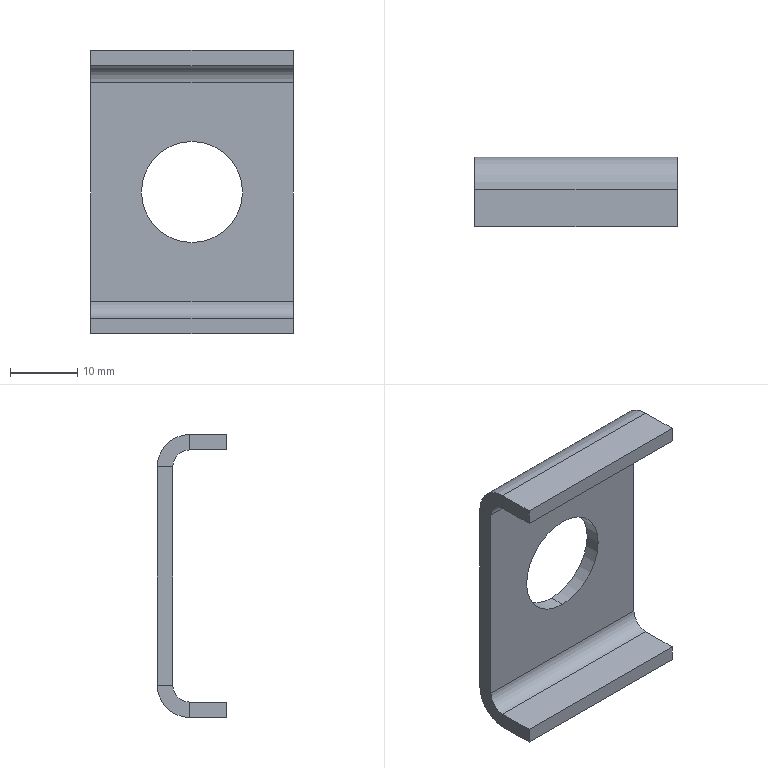Part | SolidWorks | features FlatPattern 1, ICE 1, SMBaseFlange 1, SheetMetal 1 | 1 solid | 24 faces | box 30 x 10.3 x 42 mm | volume 3379 mm3 | plane 18 | cylinder 6 | commonest cylinder face diameters 5 x2 9.6 x2 15 x2
STEP:
#1=CARTESIAN_POINT('',(15.,8.,-13.5));
#2=VERTEX_POINT('',#1);
#3=CARTESIAN_POINT('',(15.,8.,-28.5));
#4=VERTEX_POINT('',#3);
#5=CARTESIAN_POINT('',(15.,8.,-21.));
#6=DIRECTION('',(0.,-1.,0.));
#7=DIRECTION('',(0.,0.,1.));
#8=AXIS2_PLACEMENT_3D('',#5,#6,#7);
#9=CIRCLE('',#8,7.5);
#10=EDGE_CURVE('',#2,#4,#9,.T.);
#11=ORIENTED_EDGE('',*,*,#10,.T.);
#12=CARTESIAN_POINT('',(15.,10.3,-28.5));
#13=VERTEX_POINT('',#12);
#14=CARTESIAN_POINT('',(15.,-0.001,-28.5));
#15=DIRECTION('',(0.,1.,0.));
#16=VECTOR('',#15,1000.);
#17=LINE('',#14,#16);
#18=EDGE_CURVE('',#4,#13,#17,.T.);
#19=ORIENTED_EDGE('',*,*,#18,.T.);
#20=CARTESIAN_POINT('',(15.,10.3,-13.5));
#21=VERTEX_POINT('',#20);
#22=CARTESIAN_POINT('',(15.,10.3,-21.));
#23=DIRECTION('',(0.,1.,0.));
#24=DIRECTION('',(0.,0.,1.));
#25=AXIS2_PLACEMENT_3D('',#22,#23,#24);
#26=CIRCLE('',#25,7.5);
#27=EDGE_CURVE('',#13,#21,#26,.T.);
#28=ORIENTED_EDGE('',*,*,#27,.T.);
#29=CARTESIAN_POINT('',(15.,-0.001,-13.5));
#30=DIRECTION('',(0.,1.,0.));
#31=VECTOR('',#30,1000.);
#32=LINE('',#29,#31);
#33=EDGE_CURVE('',#2,#21,#32,.T.);
#34=ORIENTED_EDGE('',*,*,#33,.F.);
#35=EDGE_LOOP('',(#11,#19,#28,#34));
#36=FACE_OUTER_BOUND('',#35,.T.);
#37=CARTESIAN_POINT('',(15.,-0.001,-21.));
#38=DIRECTION('',(0.,1.,0.));
#39=DIRECTION('',(0.,0.,1.));
#40=AXIS2_PLACEMENT_3D('',#37,#38,#39);
#41=CYLINDRICAL_SURFACE('',#40,7.5);
#42=ADVANCED_FACE('',(#36),#41,.F.);
#43=CARTESIAN_POINT('',(30.,10.3,-4.8));
#44=VERTEX_POINT('',#43);
#45=CARTESIAN_POINT('',(30.,8.,-4.8));
#46=VERTEX_POINT('',#45);
#47=CARTESIAN_POINT('',(30.,10.3,-4.8));
#48=DIRECTION('',(0.,-1.,0.));
#49=VECTOR('',#48,1000.);
#50=LINE('',#47,#49);
#51=EDGE_CURVE('',#44,#46,#50,.T.);
#52=ORIENTED_EDGE('',*,*,#51,.F.);
#53=CARTESIAN_POINT('',(30.,5.5,0.));
#54=VERTEX_POINT('',#53);
#55=CARTESIAN_POINT('',(30.,5.5,-4.8));
#56=DIRECTION('',(-1.,0.,0.));
#57=DIRECTION('',(0.,0.,-1.));
#58=AXIS2_PLACEMENT_3D('',#55,#56,#57);
#59=CIRCLE('',#58,4.8);
#60=EDGE_CURVE('',#54,#44,#59,.T.);
#61=ORIENTED_EDGE('',*,*,#60,.F.);
#62=CARTESIAN_POINT('',(30.,5.5,-2.3));
#63=VERTEX_POINT('',#62);
#64=CARTESIAN_POINT('',(30.,5.5,-2.3));
#65=DIRECTION('',(0.,0.,1.));
#66=VECTOR('',#65,1000.);
#67=LINE('',#64,#66);
#68=EDGE_CURVE('',#63,#54,#67,.T.);
#69=ORIENTED_EDGE('',*,*,#68,.F.);
#70=CARTESIAN_POINT('',(30.,5.5,-4.8));
#71=DIRECTION('',(-1.,0.,0.));
#72=DIRECTION('',(0.,0.,-1.));
#73=AXIS2_PLACEMENT_3D('',#70,#71,#72);
#74=CIRCLE('',#73,2.5);
#75=EDGE_CURVE('',#63,#46,#74,.T.);
#76=ORIENTED_EDGE('',*,*,#75,.T.);
#77=EDGE_LOOP('',(#52,#61,#69,#76));
#78=FACE_OUTER_BOUND('',#77,.T.);
#79=CARTESIAN_POINT('',(30.,10.3,-4.8));
#80=DIRECTION('',(1.,0.,0.));
#81=DIRECTION('',(0.,0.,-1.));
#82=AXIS2_PLACEMENT_3D('',#79,#80,#81);
#83=PLANE('',#82);
#84=ADVANCED_FACE('',(#78),#83,.T.);
#85=CARTESIAN_POINT('',(30.,10.3,-37.2));
#86=VERTEX_POINT('',#85);
#87=CARTESIAN_POINT('',(30.,10.3,0.));
#88=DIRECTION('',(0.,0.,-1.));
#89=VECTOR('',#88,1000.);
#90=LINE('',#87,#89);
#91=EDGE_CURVE('',#44,#86,#90,.T.);
#92=ORIENTED_EDGE('',*,*,#91,.F.);
#93=ORIENTED_EDGE('',*,*,#51,.T.);
#94=CARTESIAN_POINT('',(30.,8.,-37.2));
#95=VERTEX_POINT('',#94);
#96=CARTESIAN_POINT('',(30.,8.,0.));
#97=DIRECTION('',(0.,0.,-1.));
#98=VECTOR('',#97,1000.);
#99=LINE('',#96,#98);
#100=EDGE_CURVE('',#46,#95,#99,.T.);
#101=ORIENTED_EDGE('',*,*,#100,.T.);
#102=CARTESIAN_POINT('',(30.,8.,-37.2));
#103=DIRECTION('',(0.,1.,0.));
#104=VECTOR('',#103,1000.);
#105=LINE('',#102,#104);
#106=EDGE_CURVE('',#95,#86,#105,.T.);
#107=ORIENTED_EDGE('',*,*,#106,.T.);
#108=EDGE_LOOP('',(#92,#93,#101,#107));
#109=FACE_OUTER_BOUND('',#108,.T.);
#110=CARTESIAN_POINT('',(30.,5.5,-2.3));
#111=DIRECTION('',(1.,0.,0.));
#112=DIRECTION('',(0.,0.,-1.));
#113=AXIS2_PLACEMENT_3D('',#110,#111,#112);
#114=PLANE('',#113);
#115=ADVANCED_FACE('',(#109),#114,.T.);
#116=CARTESIAN_POINT('',(0.,5.5,0.));
#117=VERTEX_POINT('',#116);
#118=CARTESIAN_POINT('',(0.,5.5,-2.3));
#119=VERTEX_POINT('',#118);
#120=CARTESIAN_POINT('',(0.,5.5,0.));
#121=DIRECTION('',(0.,0.,-1.));
#122=VECTOR('',#121,1000.);
#123=LINE('',#120,#122);
#124=EDGE_CURVE('',#117,#119,#123,.T.);
#125=ORIENTED_EDGE('',*,*,#124,.F.);
#126=CARTESIAN_POINT('',(0.,10.3,-4.8));
#127=VERTEX_POINT('',#126);
#128=CARTESIAN_POINT('',(0.,5.5,-4.8));
#129=DIRECTION('',(-1.,0.,0.));
#130=DIRECTION('',(0.,0.,-1.));
#131=AXIS2_PLACEMENT_3D('',#128,#129,#130);
#132=CIRCLE('',#131,4.8);
#133=EDGE_CURVE('',#117,#127,#132,.T.);
#134=ORIENTED_EDGE('',*,*,#133,.T.);
#135=CARTESIAN_POINT('',(0.,8.,-4.8));
#136=VERTEX_POINT('',#135);
#137=CARTESIAN_POINT('',(0.,8.,-4.8));
#138=DIRECTION('',(0.,1.,0.));
#139=VECTOR('',#138,1000.);
#140=LINE('',#137,#139);
#141=EDGE_CURVE('',#136,#127,#140,.T.);
#142=ORIENTED_EDGE('',*,*,#141,.F.);
#143=CARTESIAN_POINT('',(0.,5.5,-4.8));
#144=DIRECTION('',(-1.,0.,0.));
#145=DIRECTION('',(0.,0.,-1.));
#146=AXIS2_PLACEMENT_3D('',#143,#144,#145);
#147=CIRCLE('',#146,2.5);
#148=EDGE_CURVE('',#119,#136,#147,.T.);
#149=ORIENTED_EDGE('',*,*,#148,.F.);
#150=EDGE_LOOP('',(#125,#134,#142,#149));
#151=FACE_OUTER_BOUND('',#150,.T.);
#152=CARTESIAN_POINT('',(0.,5.5,0.));
#153=DIRECTION('',(-1.,0.,0.));
#154=DIRECTION('',(0.,0.,1.));
#155=AXIS2_PLACEMENT_3D('',#152,#153,#154);
#156=PLANE('',#155);
#157=ADVANCED_FACE('',(#151),#156,.T.);
#158=CARTESIAN_POINT('',(0.,0.,0.));
#159=VERTEX_POINT('',#158);
#160=CARTESIAN_POINT('',(0.,0.,0.));
#161=DIRECTION('',(0.,1.,0.));
#162=VECTOR('',#161,1000.);
#163=LINE('',#160,#162);
#164=EDGE_CURVE('',#159,#117,#163,.T.);
#165=ORIENTED_EDGE('',*,*,#164,.T.);
#166=ORIENTED_EDGE('',*,*,#124,.T.);
#167=CARTESIAN_POINT('',(0.,0.,-2.3));
#168=VERTEX_POINT('',#167);
#169=CARTESIAN_POINT('',(0.,0.,-2.3));
#170=DIRECTION('',(0.,1.,0.));
#171=VECTOR('',#170,1000.);
#172=LINE('',#169,#171);
#173=EDGE_CURVE('',#168,#119,#172,.T.);
#174=ORIENTED_EDGE('',*,*,#173,.F.);
#175=CARTESIAN_POINT('',(0.,0.,-2.3));
#176=DIRECTION('',(0.,0.,1.));
#177=VECTOR('',#176,1000.);
#178=LINE('',#175,#177);
#179=EDGE_CURVE('',#168,#159,#178,.T.);
#180=ORIENTED_EDGE('',*,*,#179,.T.);
#181=EDGE_LOOP('',(#165,#166,#174,#180));
#182=FACE_OUTER_BOUND('',#181,.T.);
#183=CARTESIAN_POINT('',(0.,8.,-4.8));
#184=DIRECTION('',(-1.,0.,0.));
#185=DIRECTION('',(0.,0.,1.));
#186=AXIS2_PLACEMENT_3D('',#183,#184,#185);
#187=PLANE('',#186);
#188=ADVANCED_FACE('',(#182),#187,.T.);
#189=CARTESIAN_POINT('',(30.,5.5,-42.));
#190=VERTEX_POINT('',#189);
#191=CARTESIAN_POINT('',(30.,5.5,-39.7));
#192=VERTEX_POINT('',#191);
#193=CARTESIAN_POINT('',(30.,5.5,-42.));
#194=DIRECTION('',(0.,0.,1.));
#195=VECTOR('',#194,1000.);
#196=LINE('',#193,#195);
#197=EDGE_CURVE('',#190,#192,#196,.T.);
#198=ORIENTED_EDGE('',*,*,#197,.F.);
#199=CARTESIAN_POINT('',(30.,5.5,-37.2));
#200=DIRECTION('',(-1.,0.,0.));
#201=DIRECTION('',(0.,0.,-1.));
#202=AXIS2_PLACEMENT_3D('',#199,#200,#201);
#203=CIRCLE('',#202,4.8);
#204=EDGE_CURVE('',#86,#190,#203,.T.);
#205=ORIENTED_EDGE('',*,*,#204,.F.);
#206=ORIENTED_EDGE('',*,*,#106,.F.);
#207=CARTESIAN_POINT('',(30.,5.5,-37.2));
#208=DIRECTION('',(-1.,0.,0.));
#209=DIRECTION('',(0.,0.,-1.));
#210=AXIS2_PLACEMENT_3D('',#207,#208,#209);
#211=CIRCLE('',#210,2.5);
#212=EDGE_CURVE('',#95,#192,#211,.T.);
#213=ORIENTED_EDGE('',*,*,#212,.T.);
#214=EDGE_LOOP('',(#198,#205,#206,#213));
#215=FACE_OUTER_BOUND('',#214,.T.);
#216=CARTESIAN_POINT('',(30.,5.5,-42.));
#217=DIRECTION('',(1.,0.,0.));
#218=DIRECTION('',(0.,0.,-1.));
#219=AXIS2_PLACEMENT_3D('',#216,#217,#218);
#220=PLANE('',#219);
#221=ADVANCED_FACE('',(#215),#220,.T.);
#222=CARTESIAN_POINT('',(30.,0.,-42.));
#223=VERTEX_POINT('',#222);
#224=CARTESIAN_POINT('',(30.,10.3,-42.));
#225=DIRECTION('',(0.,-1.,0.));
#226=VECTOR('',#225,1000.);
#227=LINE('',#224,#226);
#228=EDGE_CURVE('',#190,#223,#227,.T.);
#229=ORIENTED_EDGE('',*,*,#228,.F.);
#230=ORIENTED_EDGE('',*,*,#197,.T.);
#231=CARTESIAN_POINT('',(30.,0.,-39.7));
#232=VERTEX_POINT('',#231);
#233=CARTESIAN_POINT('',(30.,10.3,-39.7));
#234=DIRECTION('',(0.,-1.,0.));
#235=VECTOR('',#234,1000.);
#236=LINE('',#233,#235);
#237=EDGE_CURVE('',#192,#232,#236,.T.);
#238=ORIENTED_EDGE('',*,*,#237,.T.);
#239=CARTESIAN_POINT('',(30.,0.,-42.));
#240=DIRECTION('',(0.,0.,1.));
#241=VECTOR('',#240,1000.);
#242=LINE('',#239,#241);
#243=EDGE_CURVE('',#223,#232,#242,.T.);
#244=ORIENTED_EDGE('',*,*,#243,.F.);
#245=EDGE_LOOP('',(#229,#230,#238,#244));
#246=FACE_OUTER_BOUND('',#245,.T.);
#247=CARTESIAN_POINT('',(30.,8.,-37.2));
#248=DIRECTION('',(1.,0.,0.));
#249=DIRECTION('',(0.,0.,-1.));
#250=AXIS2_PLACEMENT_3D('',#247,#248,#249);
#251=PLANE('',#250);
#252=ADVANCED_FACE('',(#246),#251,.T.);
#253=CARTESIAN_POINT('',(0.,10.3,-37.2));
#254=VERTEX_POINT('',#253);
#255=CARTESIAN_POINT('',(0.,8.,-37.2));
#256=VERTEX_POINT('',#255);
#257=CARTESIAN_POINT('',(0.,10.3,-37.2));
#258=DIRECTION('',(0.,-1.,0.));
#259=VECTOR('',#258,1000.);
#260=LINE('',#257,#259);
#261=EDGE_CURVE('',#254,#256,#260,.T.);
#262=ORIENTED_EDGE('',*,*,#261,.F.);
#263=CARTESIAN_POINT('',(0.,5.5,-42.));
#264=VERTEX_POINT('',#263);
#265=CARTESIAN_POINT('',(0.,5.5,-37.2));
#266=DIRECTION('',(-1.,0.,0.));
#267=DIRECTION('',(0.,0.,-1.));
#268=AXIS2_PLACEMENT_3D('',#265,#266,#267);
#269=CIRCLE('',#268,4.8);
#270=EDGE_CURVE('',#254,#264,#269,.T.);
#271=ORIENTED_EDGE('',*,*,#270,.T.);
#272=CARTESIAN_POINT('',(0.,5.5,-39.7));
#273=VERTEX_POINT('',#272);
#274=CARTESIAN_POINT('',(0.,5.5,-39.7));
#275=DIRECTION('',(0.,0.,-1.));
#276=VECTOR('',#275,1000.);
#277=LINE('',#274,#276);
#278=EDGE_CURVE('',#273,#264,#277,.T.);
#279=ORIENTED_EDGE('',*,*,#278,.F.);
#280=CARTESIAN_POINT('',(0.,5.5,-37.2));
#281=DIRECTION('',(-1.,0.,0.));
#282=DIRECTION('',(0.,0.,-1.));
#283=AXIS2_PLACEMENT_3D('',#280,#281,#282);
#284=CIRCLE('',#283,2.5);
#285=EDGE_CURVE('',#256,#273,#284,.T.);
#286=ORIENTED_EDGE('',*,*,#285,.F.);
#287=EDGE_LOOP('',(#262,#271,#279,#286));
#288=FACE_OUTER_BOUND('',#287,.T.);
#289=CARTESIAN_POINT('',(0.,10.3,-37.2));
#290=DIRECTION('',(-1.,0.,0.));
#291=DIRECTION('',(0.,0.,1.));
#292=AXIS2_PLACEMENT_3D('',#289,#290,#291);
#293=PLANE('',#292);
#294=ADVANCED_FACE('',(#288),#293,.T.);
#295=CARTESIAN_POINT('',(0.,10.3,0.));
#296=DIRECTION('',(0.,0.,-1.));
#297=VECTOR('',#296,1000.);
#298=LINE('',#295,#297);
#299=EDGE_CURVE('',#127,#254,#298,.T.);
#300=ORIENTED_EDGE('',*,*,#299,.T.);
#301=ORIENTED_EDGE('',*,*,#261,.T.);
#302=CARTESIAN_POINT('',(0.,8.,0.));
#303=DIRECTION('',(0.,0.,-1.));
#304=VECTOR('',#303,1000.);
#305=LINE('',#302,#304);
#306=EDGE_CURVE('',#136,#256,#305,.T.);
#307=ORIENTED_EDGE('',*,*,#306,.F.);
#308=ORIENTED_EDGE('',*,*,#141,.T.);
#309=EDGE_LOOP('',(#300,#301,#307,#308));
#310=FACE_OUTER_BOUND('',#309,.T.);
#311=CARTESIAN_POINT('',(0.,5.5,-39.7));
#312=DIRECTION('',(-1.,0.,0.));
#313=DIRECTION('',(0.,0.,1.));
#314=AXIS2_PLACEMENT_3D('',#311,#312,#313);
#315=PLANE('',#314);
#316=ADVANCED_FACE('',(#310),#315,.T.);
#317=CARTESIAN_POINT('',(0.,0.,-39.7));
#318=VERTEX_POINT('',#317);
#319=CARTESIAN_POINT('',(0.,10.3,-39.7));
#320=DIRECTION('',(0.,-1.,0.));
#321=VECTOR('',#320,1000.);
#322=LINE('',#319,#321);
#323=EDGE_CURVE('',#273,#318,#322,.T.);
#324=ORIENTED_EDGE('',*,*,#323,.T.);
#325=CARTESIAN_POINT('',(30.,0.,-39.7));
#326=DIRECTION('',(-1.,0.,0.));
#327=VECTOR('',#326,1000.);
#328=LINE('',#325,#327);
#329=EDGE_CURVE('',#232,#318,#328,.T.);
#330=ORIENTED_EDGE('',*,*,#329,.F.);
#331=ORIENTED_EDGE('',*,*,#237,.F.);
#332=CARTESIAN_POINT('',(30.,5.5,-39.7));
#333=DIRECTION('',(-1.,0.,0.));
#334=VECTOR('',#333,1000.);
#335=LINE('',#332,#334);
#336=EDGE_CURVE('',#192,#273,#335,.T.);
#337=ORIENTED_EDGE('',*,*,#336,.T.);
#338=EDGE_LOOP('',(#324,#330,#331,#337));
#339=FACE_OUTER_BOUND('',#338,.T.);
#340=CARTESIAN_POINT('',(30.,10.3,-39.7));
#341=DIRECTION('',(0.,0.,-1.));
#342=DIRECTION('',(-1.,0.,0.));
#343=AXIS2_PLACEMENT_3D('',#340,#341,#342);
#344=PLANE('',#343);
#345=ADVANCED_FACE('',(#339),#344,.F.);
#346=CARTESIAN_POINT('',(0.,0.,-42.));
#347=VERTEX_POINT('',#346);
#348=CARTESIAN_POINT('',(0.,0.,-42.));
#349=DIRECTION('',(0.,0.,1.));
#350=VECTOR('',#349,1000.);
#351=LINE('',#348,#350);
#352=EDGE_CURVE('',#347,#318,#351,.T.);
#353=ORIENTED_EDGE('',*,*,#352,.F.);
#354=CARTESIAN_POINT('',(30.,0.,-42.));
#355=DIRECTION('',(-1.,0.,0.));
#356=VECTOR('',#355,1000.);
#357=LINE('',#354,#356);
#358=EDGE_CURVE('',#223,#347,#357,.T.);
#359=ORIENTED_EDGE('',*,*,#358,.F.);
#360=ORIENTED_EDGE('',*,*,#243,.T.);
#361=ORIENTED_EDGE('',*,*,#329,.T.);
#362=EDGE_LOOP('',(#353,#359,#360,#361));
#363=FACE_OUTER_BOUND('',#362,.T.);
#364=CARTESIAN_POINT('',(30.,0.,-42.));
#365=DIRECTION('',(0.,-1.,0.));
#366=DIRECTION('',(0.,0.,-1.));
#367=AXIS2_PLACEMENT_3D('',#364,#365,#366);
#368=PLANE('',#367);
#369=ADVANCED_FACE('',(#363),#368,.T.);
#370=CARTESIAN_POINT('',(0.,10.3,-42.));
#371=DIRECTION('',(0.,-1.,0.));
#372=VECTOR('',#371,1000.);
#373=LINE('',#370,#372);
#374=EDGE_CURVE('',#264,#347,#373,.T.);
#375=ORIENTED_EDGE('',*,*,#374,.F.);
#376=CARTESIAN_POINT('',(30.,5.5,-42.));
#377=DIRECTION('',(-1.,0.,0.));
#378=VECTOR('',#377,1000.);
#379=LINE('',#376,#378);
#380=EDGE_CURVE('',#190,#264,#379,.T.);
#381=ORIENTED_EDGE('',*,*,#380,.F.);
#382=ORIENTED_EDGE('',*,*,#228,.T.);
#383=ORIENTED_EDGE('',*,*,#358,.T.);
#384=EDGE_LOOP('',(#375,#381,#382,#383));
#385=FACE_OUTER_BOUND('',#384,.T.);
#386=CARTESIAN_POINT('',(30.,10.3,-42.));
#387=DIRECTION('',(0.,0.,-1.));
#388=DIRECTION('',(-1.,0.,0.));
#389=AXIS2_PLACEMENT_3D('',#386,#387,#388);
#390=PLANE('',#389);
#391=ADVANCED_FACE('',(#385),#390,.T.);
#392=ORIENTED_EDGE('',*,*,#270,.F.);
#393=CARTESIAN_POINT('',(30.,10.3,-37.2));
#394=DIRECTION('',(-1.,0.,0.));
#395=VECTOR('',#394,1000.);
#396=LINE('',#393,#395);
#397=EDGE_CURVE('',#86,#254,#396,.T.);
#398=ORIENTED_EDGE('',*,*,#397,.F.);
#399=ORIENTED_EDGE('',*,*,#204,.T.);
#400=ORIENTED_EDGE('',*,*,#380,.T.);
#401=EDGE_LOOP('',(#392,#398,#399,#400));
#402=FACE_OUTER_BOUND('',#401,.T.);
#403=CARTESIAN_POINT('',(30.,5.5,-37.2));
#404=DIRECTION('',(-1.,0.,0.));
#405=DIRECTION('',(0.,0.,1.));
#406=AXIS2_PLACEMENT_3D('',#403,#404,#405);
#407=CYLINDRICAL_SURFACE('',#406,4.8);
#408=ADVANCED_FACE('',(#402),#407,.T.);
#409=CARTESIAN_POINT('',(15.,10.3,-21.));
#410=DIRECTION('',(0.,1.,0.));
#411=DIRECTION('',(0.,0.,1.));
#412=AXIS2_PLACEMENT_3D('',#409,#410,#411);
#413=CIRCLE('',#412,7.5);
#414=EDGE_CURVE('',#21,#13,#413,.T.);
#415=ORIENTED_EDGE('',*,*,#414,.F.);
#416=ORIENTED_EDGE('',*,*,#27,.F.);
#417=EDGE_LOOP('',(#415,#416));
#418=FACE_BOUND('',#417,.T.);
#419=ORIENTED_EDGE('',*,*,#299,.F.);
#420=CARTESIAN_POINT('',(30.,10.3,-4.8));
#421=DIRECTION('',(-1.,0.,0.));
#422=VECTOR('',#421,1000.);
#423=LINE('',#420,#422);
#424=EDGE_CURVE('',#44,#127,#423,.T.);
#425=ORIENTED_EDGE('',*,*,#424,.F.);
#426=ORIENTED_EDGE('',*,*,#91,.T.);
#427=ORIENTED_EDGE('',*,*,#397,.T.);
#428=EDGE_LOOP('',(#419,#425,#426,#427));
#429=FACE_OUTER_BOUND('',#428,.T.);
#430=CARTESIAN_POINT('',(30.,10.3,0.));
#431=DIRECTION('',(0.,1.,0.));
#432=DIRECTION('',(0.,0.,1.));
#433=AXIS2_PLACEMENT_3D('',#430,#431,#432);
#434=PLANE('',#433);
#435=ADVANCED_FACE('',(#418,#429),#434,.T.);
#436=ORIENTED_EDGE('',*,*,#133,.F.);
#437=CARTESIAN_POINT('',(30.,5.5,0.));
#438=DIRECTION('',(-1.,0.,0.));
#439=VECTOR('',#438,1000.);
#440=LINE('',#437,#439);
#441=EDGE_CURVE('',#54,#117,#440,.T.);
#442=ORIENTED_EDGE('',*,*,#441,.F.);
#443=ORIENTED_EDGE('',*,*,#60,.T.);
#444=ORIENTED_EDGE('',*,*,#424,.T.);
#445=EDGE_LOOP('',(#436,#442,#443,#444));
#446=FACE_OUTER_BOUND('',#445,.T.);
#447=CARTESIAN_POINT('',(30.,5.5,-4.8));
#448=DIRECTION('',(-1.,0.,0.));
#449=DIRECTION('',(0.,0.,1.));
#450=AXIS2_PLACEMENT_3D('',#447,#448,#449);
#451=CYLINDRICAL_SURFACE('',#450,4.8);
#452=ADVANCED_FACE('',(#446),#451,.T.);
#453=ORIENTED_EDGE('',*,*,#164,.F.);
#454=CARTESIAN_POINT('',(30.,0.,0.));
#455=VERTEX_POINT('',#454);
#456=CARTESIAN_POINT('',(30.,0.,0.));
#457=DIRECTION('',(-1.,0.,0.));
#458=VECTOR('',#457,1000.);
#459=LINE('',#456,#458);
#460=EDGE_CURVE('',#455,#159,#459,.T.);
#461=ORIENTED_EDGE('',*,*,#460,.F.);
#462=CARTESIAN_POINT('',(30.,0.,0.));
#463=DIRECTION('',(0.,1.,0.));
#464=VECTOR('',#463,1000.);
#465=LINE('',#462,#464);
#466=EDGE_CURVE('',#455,#54,#465,.T.);
#467=ORIENTED_EDGE('',*,*,#466,.T.);
#468=ORIENTED_EDGE('',*,*,#441,.T.);
#469=EDGE_LOOP('',(#453,#461,#467,#468));
#470=FACE_OUTER_BOUND('',#469,.T.);
#471=CARTESIAN_POINT('',(30.,0.,0.));
#472=DIRECTION('',(0.,0.,1.));
#473=DIRECTION('',(1.,0.,0.));
#474=AXIS2_PLACEMENT_3D('',#471,#472,#473);
#475=PLANE('',#474);
#476=ADVANCED_FACE('',(#470),#475,.T.);
#477=ORIENTED_EDGE('',*,*,#179,.F.);
#478=CARTESIAN_POINT('',(30.,0.,-2.3));
#479=VERTEX_POINT('',#478);
#480=CARTESIAN_POINT('',(30.,0.,-2.3));
#481=DIRECTION('',(-1.,0.,0.));
#482=VECTOR('',#481,1000.);
#483=LINE('',#480,#482);
#484=EDGE_CURVE('',#479,#168,#483,.T.);
#485=ORIENTED_EDGE('',*,*,#484,.F.);
#486=CARTESIAN_POINT('',(30.,0.,-2.3));
#487=DIRECTION('',(0.,0.,1.));
#488=VECTOR('',#487,1000.);
#489=LINE('',#486,#488);
#490=EDGE_CURVE('',#479,#455,#489,.T.);
#491=ORIENTED_EDGE('',*,*,#490,.T.);
#492=ORIENTED_EDGE('',*,*,#460,.T.);
#493=EDGE_LOOP('',(#477,#485,#491,#492));
#494=FACE_OUTER_BOUND('',#493,.T.);
#495=CARTESIAN_POINT('',(30.,0.,-2.3));
#496=DIRECTION('',(0.,-1.,0.));
#497=DIRECTION('',(0.,0.,-1.));
#498=AXIS2_PLACEMENT_3D('',#495,#496,#497);
#499=PLANE('',#498);
#500=ADVANCED_FACE('',(#494),#499,.T.);
#501=ORIENTED_EDGE('',*,*,#173,.T.);
#502=CARTESIAN_POINT('',(30.,5.5,-2.3));
#503=DIRECTION('',(-1.,0.,0.));
#504=VECTOR('',#503,1000.);
#505=LINE('',#502,#504);
#506=EDGE_CURVE('',#63,#119,#505,.T.);
#507=ORIENTED_EDGE('',*,*,#506,.F.);
#508=CARTESIAN_POINT('',(30.,0.,-2.3));
#509=DIRECTION('',(0.,1.,0.));
#510=VECTOR('',#509,1000.);
#511=LINE('',#508,#510);
#512=EDGE_CURVE('',#479,#63,#511,.T.);
#513=ORIENTED_EDGE('',*,*,#512,.F.);
#514=ORIENTED_EDGE('',*,*,#484,.T.);
#515=EDGE_LOOP('',(#501,#507,#513,#514));
#516=FACE_OUTER_BOUND('',#515,.T.);
#517=CARTESIAN_POINT('',(30.,0.,-2.3));
#518=DIRECTION('',(0.,0.,1.));
#519=DIRECTION('',(1.,0.,0.));
#520=AXIS2_PLACEMENT_3D('',#517,#518,#519);
#521=PLANE('',#520);
#522=ADVANCED_FACE('',(#516),#521,.F.);
#523=ORIENTED_EDGE('',*,*,#148,.T.);
#524=CARTESIAN_POINT('',(30.,8.,-4.8));
#525=DIRECTION('',(-1.,0.,0.));
#526=VECTOR('',#525,1000.);
#527=LINE('',#524,#526);
#528=EDGE_CURVE('',#46,#136,#527,.T.);
#529=ORIENTED_EDGE('',*,*,#528,.F.);
#530=ORIENTED_EDGE('',*,*,#75,.F.);
#531=ORIENTED_EDGE('',*,*,#506,.T.);
#532=EDGE_LOOP('',(#523,#529,#530,#531));
#533=FACE_OUTER_BOUND('',#532,.T.);
#534=CARTESIAN_POINT('',(30.,5.5,-4.8));
#535=DIRECTION('',(-1.,0.,0.));
#536=DIRECTION('',(0.,0.,1.));
#537=AXIS2_PLACEMENT_3D('',#534,#535,#536);
#538=CYLINDRICAL_SURFACE('',#537,2.5);
#539=ADVANCED_FACE('',(#533),#538,.F.);
#540=ORIENTED_EDGE('',*,*,#10,.F.);
#541=CARTESIAN_POINT('',(15.,8.,-21.));
#542=DIRECTION('',(0.,-1.,0.));
#543=DIRECTION('',(0.,0.,1.));
#544=AXIS2_PLACEMENT_3D('',#541,#542,#543);
#545=CIRCLE('',#544,7.5);
#546=EDGE_CURVE('',#4,#2,#545,.T.);
#547=ORIENTED_EDGE('',*,*,#546,.F.);
#548=EDGE_LOOP('',(#540,#547));
#549=FACE_BOUND('',#548,.T.);
#550=ORIENTED_EDGE('',*,*,#306,.T.);
#551=CARTESIAN_POINT('',(30.,8.,-37.2));
#552=DIRECTION('',(-1.,0.,0.));
#553=VECTOR('',#552,1000.);
#554=LINE('',#551,#553);
#555=EDGE_CURVE('',#95,#256,#554,.T.);
#556=ORIENTED_EDGE('',*,*,#555,.F.);
#557=ORIENTED_EDGE('',*,*,#100,.F.);
#558=ORIENTED_EDGE('',*,*,#528,.T.);
#559=EDGE_LOOP('',(#550,#556,#557,#558));
#560=FACE_OUTER_BOUND('',#559,.T.);
#561=CARTESIAN_POINT('',(30.,8.,0.));
#562=DIRECTION('',(0.,1.,0.));
#563=DIRECTION('',(0.,0.,1.));
#564=AXIS2_PLACEMENT_3D('',#561,#562,#563);
#565=PLANE('',#564);
#566=ADVANCED_FACE('',(#549,#560),#565,.F.);
#567=ORIENTED_EDGE('',*,*,#285,.T.);
#568=ORIENTED_EDGE('',*,*,#336,.F.);
#569=ORIENTED_EDGE('',*,*,#212,.F.);
#570=ORIENTED_EDGE('',*,*,#555,.T.);
#571=EDGE_LOOP('',(#567,#568,#569,#570));
#572=FACE_OUTER_BOUND('',#571,.T.);
#573=CARTESIAN_POINT('',(30.,5.5,-37.2));
#574=DIRECTION('',(-1.,0.,0.));
#575=DIRECTION('',(0.,0.,1.));
#576=AXIS2_PLACEMENT_3D('',#573,#574,#575);
#577=CYLINDRICAL_SURFACE('',#576,2.5);
#578=ADVANCED_FACE('',(#572),#577,.F.);
#579=ORIENTED_EDGE('',*,*,#512,.T.);
#580=ORIENTED_EDGE('',*,*,#68,.T.);
#581=ORIENTED_EDGE('',*,*,#466,.F.);
#582=ORIENTED_EDGE('',*,*,#490,.F.);
#583=EDGE_LOOP('',(#579,#580,#581,#582));
#584=FACE_OUTER_BOUND('',#583,.T.);
#585=CARTESIAN_POINT('',(30.,5.5,-37.2));
#586=DIRECTION('',(1.,0.,0.));
#587=DIRECTION('',(0.,0.,-1.));
#588=AXIS2_PLACEMENT_3D('',#585,#586,#587);
#589=PLANE('',#588);
#590=ADVANCED_FACE('',(#584),#589,.T.);
#591=ORIENTED_EDGE('',*,*,#323,.F.);
#592=ORIENTED_EDGE('',*,*,#278,.T.);
#593=ORIENTED_EDGE('',*,*,#374,.T.);
#594=ORIENTED_EDGE('',*,*,#352,.T.);
#595=EDGE_LOOP('',(#591,#592,#593,#594));
#596=FACE_OUTER_BOUND('',#595,.T.);
#597=CARTESIAN_POINT('',(0.,5.5,-37.2));
#598=DIRECTION('',(1.,0.,0.));
#599=DIRECTION('',(0.,0.,-1.));
#600=AXIS2_PLACEMENT_3D('',#597,#598,#599);
#601=PLANE('',#600);
#602=ADVANCED_FACE('',(#596),#601,.F.);
#603=ORIENTED_EDGE('',*,*,#18,.F.);
#604=ORIENTED_EDGE('',*,*,#546,.T.);
#605=ORIENTED_EDGE('',*,*,#33,.T.);
#606=ORIENTED_EDGE('',*,*,#414,.T.);
#607=EDGE_LOOP('',(#603,#604,#605,#606));
#608=FACE_OUTER_BOUND('',#607,.T.);
#609=CARTESIAN_POINT('',(15.,-0.001,-21.));
#610=DIRECTION('',(0.,1.,0.));
#611=DIRECTION('',(0.,0.,1.));
#612=AXIS2_PLACEMENT_3D('',#609,#610,#611);
#613=CYLINDRICAL_SURFACE('',#612,7.5);
#614=ADVANCED_FACE('',(#608),#613,.F.);
#615=CLOSED_SHELL('',(#42,#84,#115,#157,#188,#221,#252,#294,#316,#345,#369,#391,#408,#435,#452,#476,#500,#522,#539,#566,#578,#590,#602,#614));
#616=MANIFOLD_SOLID_BREP('',#615);
#617=CARTESIAN_POINT('',(0.,0.,0.));
#618=DIRECTION('',(0.,0.,1.));
#619=DIRECTION('',(1.,0.,0.));
#620=AXIS2_PLACEMENT_3D('',#617,#618,#619);
#621=(LENGTH_UNIT()NAMED_UNIT(*)SI_UNIT(.MILLI.,.METRE.));
#622=UNCERTAINTY_MEASURE_WITH_UNIT(LENGTH_MEASURE(0.00001),#621,'','');
#623=(NAMED_UNIT(*)PLANE_ANGLE_UNIT()SI_UNIT($,.RADIAN.));
#624=(NAMED_UNIT(*)SI_UNIT($,.STERADIAN.)SOLID_ANGLE_UNIT());
#625=(GEOMETRIC_REPRESENTATION_CONTEXT(3)GLOBAL_UNCERTAINTY_ASSIGNED_CONTEXT((#622))GLOBAL_UNIT_ASSIGNED_CONTEXT((#621,#623,#624))REPRESENTATION_CONTEXT('',''));
#626=ADVANCED_BREP_SHAPE_REPRESENTATION('',(#616,#620),#625);